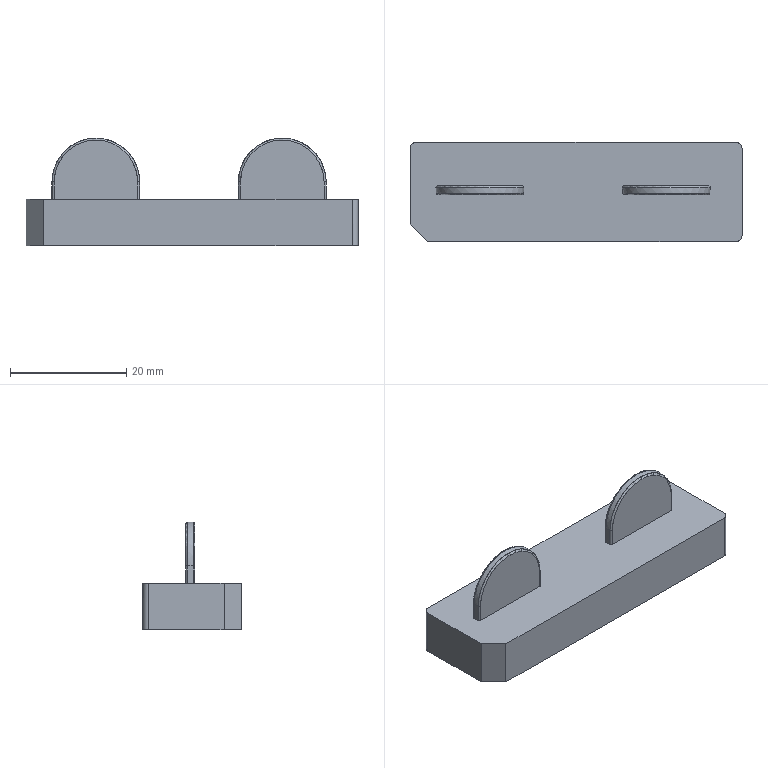NC program | PowerMill | posted by the shop | part box 57 x 17 x 18.538 mm
Lines 10661 to 11689 of 218548:
( TOOL ID   R1.5_1_1 )
( TOOL DIA. 3. TIP RAD 1.5 LENGTH 64.36 )
( Z = -9.391 )
T22 M6
T10
G91 G28 Z0
G0 G90 G54
M08
S22000 M3
X0 Y0 M8
G43 Z10.797 H22
X-10.444 Y-.885
Z-1.573
G1 Z-2.773 F1200
X-10.442 Y-.861 Z-2.798 F2000
X-10.437 Y-.836 Z-2.821
X-10.427 Y-.811 Z-2.843
X-10.415 Y-.785 Z-2.862
X-10.398 Y-.76 Z-2.88
X-10.379 Y-.736 Z-2.895
X-10.361 Y-.717 Z-2.906
X-10.33 Y-.685 Z-2.922
X-10.298 Y-.654 Z-2.94
X-10.264 Y-.62 Z-2.961
X-10.233 Y-.589 Z-2.981
X-10.203 Y-.559 Z-3.001
X-10.173 Y-.529 Z-3.023
X-10.16 Y-.515 Z-3.033
X-10.137 Y-.494 Z-3.049
X-10.111 Y-.474 Z-3.061
X-10.084 Y-.455 Z-3.07
X-10.054 Y-.438 Z-3.076
X-10.024 Y-.423 Z-3.079
X-9.992 Y-.409
X-9.966 Y-.4 Z-3.076
X-9.936 Y-.312 Z-3.091
X-9.969 Y-.324 Z-3.093
X-10. Y-.339
X-10.031 Y-.355 Z-3.089
X-10.059 Y-.372 Z-3.081
X-10.086 Y-.391 Z-3.071
X-10.111 Y-.411 Z-3.057
X-10.129 Y-.428 Z-3.044
X-10.159 Y-.458 Z-3.02
X-10.209 Y-.508 Z-2.981
X-10.266 Y-.565 Z-2.941
X-10.328 Y-.627 Z-2.901
X-10.39 Y-.689 Z-2.865
X-10.449 Y-.748 Z-2.835
X-10.504 Y-.803 Z-2.811
X-10.555 Y-.855 Z-2.791
X-10.606 Y-.905 Z-2.776
X-10.629 Y-.93 Z-2.767
X-10.649 Y-.956 Z-2.756
X-10.665 Y-.983 Z-2.742
X-10.679 Y-1.011 Z-2.726
X-10.689 Y-1.038 Z-2.708
X-10.696 Y-1.066 Z-2.689
X-10.699 Y-1.088 Z-2.672
X-10.809 Y-1.143 Z-2.618
X-10.805 Y-1.115 Z-2.638
X-10.797 Y-1.087 Z-2.656
X-10.786 Y-1.058 Z-2.672
X-10.771 Y-1.03 Z-2.686
X-10.753 Y-1.003 Z-2.697
X-10.733 Y-.977 Z-2.706
X-10.714 Y-.956 Z-2.712
X-10.662 Y-.904 Z-2.724
X-10.608 Y-.851 Z-2.741
X-10.552 Y-.795 Z-2.762
X-10.493 Y-.736 Z-2.788
X-10.432 Y-.675 Z-2.819
X-10.37 Y-.612 Z-2.855
X-10.306 Y-.549 Z-2.896
X-10.244 Y-.487 Z-2.94
X-10.186 Y-.428 Z-2.985
X-10.132 Y-.375 Z-3.031
X-10.113 Y-.356 Z-3.047
X-10.091 Y-.335 Z-3.064
X-10.066 Y-.316 Z-3.079
X-10.039 Y-.297 Z-3.09
X-10.011 Y-.28 Z-3.097
X-9.98 Y-.264 Z-3.102
X-9.949 Y-.249
X-9.923 Y-.239 Z-3.101
X-9.912 Y-.167 Z-3.109
X-9.944 Y-.181 Z-3.11
X-9.975 Y-.196 Z-3.109
X-10.005 Y-.213 Z-3.103
X-10.033 Y-.231 Z-3.095
X-10.059 Y-.25 Z-3.083
X-10.083 Y-.27 Z-3.067
X-10.1 Y-.286 Z-3.053
X-10.144 Y-.33 Z-3.013
X-10.205 Y-.391 Z-2.959
X-10.269 Y-.455 Z-2.908
X-10.332 Y-.518 Z-2.862
X-10.396 Y-.582 Z-2.82
X-10.459 Y-.645 Z-2.782
X-10.521 Y-.707 Z-2.75
X-10.582 Y-.768 Z-2.722
X-10.642 Y-.828 Z-2.698
X-10.701 Y-.887 Z-2.679
X-10.758 Y-.944 Z-2.664
X-10.814 Y-1. Z-2.653
X-10.837 Y-1.025 Z-2.647
X-10.858 Y-1.052 Z-2.639
X-10.875 Y-1.08 Z-2.628
X-10.889 Y-1.108 Z-2.615
X-10.9 Y-1.137 Z-2.599
X-10.908 Y-1.166 Z-2.582
X-10.911 Y-1.19 Z-2.567
X-11.011 Y-1.233 Z-2.525
X-11.005 Y-1.203 Z-2.542
X-10.997 Y-1.173 Z-2.558
X-10.984 Y-1.144 Z-2.571
X-10.969 Y-1.115 Z-2.582
X-10.951 Y-1.087 Z-2.591
X-10.93 Y-1.06 Z-2.597
X-10.911 Y-1.04 Z-2.6
X-10.864 Y-.993 Z-2.606
X-10.816 Y-.945 Z-2.614
X-10.763 Y-.892 Z-2.628
X-10.705 Y-.834 Z-2.646
X-10.643 Y-.772 Z-2.669
X-10.584 Y-.714 Z-2.695
X-10.533 Y-.662 Z-2.72
X-10.488 Y-.618 Z-2.745
X-10.445 Y-.574 Z-2.771
X-10.387 Y-.516 Z-2.809
X-10.329 Y-.459 Z-2.85
X-10.27 Y-.4 Z-2.896
X-10.206 Y-.336 Z-2.95
X-10.149 Y-.279 Z-3.001
X-10.096 Y-.226 Z-3.052
X-10.088 Y-.218 Z-3.059
X-10.067 Y-.198 Z-3.077
X-10.043 Y-.178 Z-3.092
X-10.016 Y-.159 Z-3.104
X-9.988 Y-.142 Z-3.112
X-9.958 Y-.125 Z-3.117
X-9.927 Y-.11 Z-3.119
X-9.901 Y-.099 Z-3.117
X-9.89 Y-.031 Z-3.119
X-9.921 Y-.045 Z-3.121
X-9.952 Y-.06 Z-3.119
X-9.982 Y-.077 Z-3.114
X-10.01 Y-.095 Z-3.105
X-10.036 Y-.114 Z-3.093
X-10.06 Y-.134 Z-3.078
X-10.078 Y-.151 Z-3.064
X-10.089 Y-.162 Z-3.053
X-10.138 Y-.211 Z-3.007
X-10.188 Y-.261 Z-2.961
X-10.242 Y-.315 Z-2.912
X-10.293 Y-.366 Z-2.868
X-10.344 Y-.417 Z-2.827
X-10.409 Y-.482 Z-2.779
X-10.473 Y-.546 Z-2.736
X-10.536 Y-.609 Z-2.698
X-10.599 Y-.672 Z-2.664
X-10.661 Y-.734 Z-2.635
X-10.722 Y-.795 Z-2.61
X-10.784 Y-.857 Z-2.589
X-10.842 Y-.914 Z-2.573
X-10.896 Y-.969 Z-2.562
X-10.948 Y-1.021 Z-2.554
X-10.998 Y-1.071 Z-2.551
X-11.022 Y-1.097 Z-2.548
X-11.042 Y-1.124 Z-2.543
X-11.06 Y-1.152 Z-2.535
X-11.075 Y-1.181 Z-2.524
X-11.087 Y-1.211 Z-2.511
X-11.096 Y-1.241 Z-2.497
X-11.1 Y-1.266 Z-2.483
X-11.185 Y-1.295 Z-2.446
X-11.179 Y-1.264 Z-2.462
X-11.169 Y-1.234 Z-2.475
X-11.157 Y-1.203 Z-2.486
X-11.141 Y-1.174 Z-2.494
X-11.122 Y-1.145 Z-2.5
X-11.101 Y-1.118 Z-2.504
X-11.082 Y-1.098
X-11.045 Y-1.061
X-11.008 Y-1.025 Z-2.507
X-10.966 Y-.982 Z-2.513
X-10.911 Y-.927 Z-2.523
X-10.867 Y-.883 Z-2.533
X-10.831 Y-.847 Z-2.543
X-10.795 Y-.811 Z-2.555
X-10.739 Y-.756 Z-2.576
X-10.685 Y-.701 Z-2.6
X-10.63 Y-.647 Z-2.627
X-10.576 Y-.592 Z-2.656
X-10.52 Y-.537 Z-2.69
X-10.464 Y-.48 Z-2.728
X-10.404 Y-.42 Z-2.771
X-10.34 Y-.357 Z-2.822
X-10.269 Y-.285 Z-2.883
X-10.186 Y-.202 Z-2.957
X-10.106 Y-.123 Z-3.032
X-10.068 Y-.084 Z-3.067
X-10.046 Y-.064 Z-3.085
X-10.022 Y-.044 Z-3.1
X-9.995 Y-.025 Z-3.111
X-9.967 Y-.007 Z-3.119
X-9.937 Y.009 Z-3.124
X-9.906 Y.024 Z-3.125
X-9.88 Y.035 Z-3.123
X-9.877 Y.095 Z-3.121
X-9.909 Y.081 Z-3.123
X-9.94 Y.066 Z-3.121
X-9.969 Y.049 Z-3.116
X-9.998 Y.031 Z-3.107
X-10.024 Y.011 Z-3.095
X-10.048 Y-.008 Z-3.08
X-10.065 Y-.025 Z-3.065
X-10.083 Y-.043 Z-3.048
X-10.126 Y-.086 Z-3.008
X-10.17 Y-.129 Z-2.968
X-10.213 Y-.173 Z-2.928
X-10.274 Y-.234 Z-2.873
X-10.329 Y-.288 Z-2.825
X-10.373 Y-.333 Z-2.788
X-10.417 Y-.377 Z-2.751
X-10.463 Y-.423 Z-2.716
X-10.509 Y-.469 Z-2.683
X-10.571 Y-.531 Z-2.642
X-10.635 Y-.595 Z-2.604
X-10.699 Y-.659 Z-2.571
X-10.763 Y-.723 Z-2.541
X-10.825 Y-.785 Z-2.517
X-10.886 Y-.846 Z-2.497
X-10.945 Y-.905 Z-2.481
X-11.002 Y-.962 Z-2.47
X-11.058 Y-1.018 Z-2.462
X-11.111 Y-1.071 Z-2.459
X-11.163 Y-1.123 Z-2.46
X-11.187 Y-1.149 Z-2.459
X-11.208 Y-1.176 Z-2.455
X-11.226 Y-1.205 Z-2.449
X-11.241 Y-1.234 Z-2.44
X-11.253 Y-1.264 Z-2.429
X-11.262 Y-1.295 Z-2.416
X-11.267 Y-1.32 Z-2.404
X-11.349 Y-1.346 Z-2.368
X-11.343 Y-1.315 Z-2.382
X-11.333 Y-1.284 Z-2.394
X-11.32 Y-1.253 Z-2.403
X-11.304 Y-1.224 Z-2.411
X-11.285 Y-1.195 Z-2.415
X-11.263 Y-1.168 Z-2.417
X-11.244 Y-1.147
X-11.194 Y-1.098 Z-2.414
X-11.143 Y-1.046 Z-2.415
X-11.089 Y-.992 Z-2.419
X-11.032 Y-.935 Z-2.428
X-10.974 Y-.877 Z-2.441
X-10.913 Y-.816 Z-2.459
X-10.851 Y-.754 Z-2.481
X-10.787 Y-.69 Z-2.508
X-10.723 Y-.626 Z-2.538
X-10.66 Y-.563 Z-2.573
X-10.613 Y-.517 Z-2.6
X-10.565 Y-.468 Z-2.632
X-10.517 Y-.42 Z-2.667
X-10.469 Y-.372 Z-2.703
X-10.417 Y-.32 Z-2.745
X-10.356 Y-.259 Z-2.796
X-10.281 Y-.184 Z-2.862
X-10.183 Y-.086 Z-2.95
X-10.113 Y-.016 Z-3.014
X-10.062 Y.035 Z-3.062
X-10.04 Y.055 Z-3.08
X-10.016 Y.074 Z-3.094
X-9.99 Y.093 Z-3.106
X-9.961 Y.111 Z-3.114
X-9.931 Y.128 Z-3.119
X-9.9 Y.143 Z-3.12
X-9.874 Y.154 Z-3.118
X-9.872 Y.213 Z-3.116
X-9.904 Y.199 Z-3.118
X-9.935 Y.184 Z-3.116
X-9.964 Y.167 Z-3.11
X-9.992 Y.149 Z-3.102
X-10.018 Y.13 Z-3.089
X-10.042 Y.11 Z-3.074
X-10.06 Y.094 Z-3.059
X-10.106 Y.048 Z-3.016
X-10.156 Y-.003 Z-2.969
X-10.207 Y-.053 Z-2.923
X-10.257 Y-.104 Z-2.878
X-10.309 Y-.155 Z-2.833
X-10.368 Y-.214 Z-2.781
X-10.419 Y-.266 Z-2.737
X-10.471 Y-.318 Z-2.694
X-10.524 Y-.37 Z-2.652
X-10.577 Y-.423 Z-2.613
X-10.641 Y-.488 Z-2.569
X-10.706 Y-.553 Z-2.53
X-10.772 Y-.618 Z-2.494
X-10.838 Y-.684 Z-2.462
X-10.89 Y-.736 Z-2.44
X-10.945 Y-.792 Z-2.42
X-11.006 Y-.852 Z-2.402
X-11.067 Y-.914 Z-2.388
X-11.125 Y-.972 Z-2.378
X-11.18 Y-1.026 Z-2.372
X-11.23 Y-1.076 Z-2.37
X-11.276 Y-1.122 Z-2.371
X-11.321 Y-1.167 Z-2.376
X-11.344 Y-1.193 Z-2.377
X-11.365 Y-1.22 Z-2.376
X-11.384 Y-1.249 Z-2.372
X-11.399 Y-1.279 Z-2.365
X-11.412 Y-1.31 Z-2.356
X-11.421 Y-1.342 Z-2.344
X-11.427 Y-1.367 Z-2.334
X-11.502 Y-1.386 Z-2.297
X-11.496 Y-1.355 Z-2.31
X-11.485 Y-1.323 Z-2.32
X-11.472 Y-1.292 Z-2.329
X-11.456 Y-1.262 Z-2.334
X-11.437 Y-1.234 Z-2.337
X-11.415 Y-1.207
X-11.396 Y-1.186 Z-2.336
X-11.35 Y-1.14 Z-2.33
X-11.303 Y-1.093 Z-2.327
X-11.251 Y-1.041 Z-2.328
X-11.195 Y-.985 Z-2.333
X-11.135 Y-.925 Z-2.341
X-11.073 Y-.864 Z-2.354
X-11.016 Y-.806 Z-2.37
X-10.963 Y-.753 Z-2.387
X-10.915 Y-.705 Z-2.406
X-10.855 Y-.645 Z-2.433
X-10.794 Y-.584 Z-2.464
X-10.729 Y-.519 Z-2.501
X-10.663 Y-.453 Z-2.542
X-10.603 Y-.393 Z-2.584
X-10.547 Y-.338 Z-2.626
X-10.493 Y-.283 Z-2.671
X-10.367 Y-.157 Z-2.777
X-10.24 Y-.03 Z-2.888
X-10.111 Y.099 Z-3.006
X-10.057 Y.153 Z-3.057
X-10.035 Y.173 Z-3.074
X-10.011 Y.193 Z-3.089
X-9.984 Y.212 Z-3.101
X-9.956 Y.23 Z-3.109
X-9.926 Y.246 Z-3.113
X-9.895 Y.261 Z-3.115
X-9.869 Y.272 Z-3.113
X-9.867 Y.331 Z-3.111
X-9.898 Y.318 Z-3.113
X-9.929 Y.302 Z-3.111
X-9.959 Y.285 Z-3.105
X-9.987 Y.267 Z-3.096
X-10.013 Y.248 Z-3.084
X-10.037 Y.228 Z-3.068
X-10.054 Y.212 Z-3.054
X-10.07 Y.197 Z-3.039
X-10.121 Y.145 Z-2.991
X-10.172 Y.094 Z-2.944
X-10.224 Y.042 Z-2.897
X-10.276 Y-.01 Z-2.851
X-10.347 Y-.081 Z-2.789
X-10.427 Y-.161 Z-2.72
X-10.486 Y-.219 Z-2.671
X-10.539 Y-.272 Z-2.628
X-10.592 Y-.326 Z-2.585
X-10.646 Y-.38 Z-2.545
X-10.693 Y-.426 Z-2.511
X-10.756 Y-.489 Z-2.47
X-10.82 Y-.553 Z-2.433
X-10.884 Y-.618 Z-2.399
X-10.948 Y-.682 Z-2.37
X-11.012 Y-.745 Z-2.345
X-11.074 Y-.808 Z-2.325
X-11.135 Y-.869 Z-2.309
X-11.195 Y-.928 Z-2.297
X-11.253 Y-.987 Z-2.289
X-11.31 Y-1.043 Z-2.285
X-11.365 Y-1.098
X-11.418 Y-1.152 Z-2.289
X-11.47 Y-1.204 Z-2.297
X-11.494 Y-1.229 Z-2.299
X-11.515 Y-1.257
X-11.533 Y-1.286 Z-2.296
X-11.549 Y-1.316 Z-2.291
X-11.562 Y-1.347 Z-2.283
X-11.572 Y-1.379 Z-2.272
X-11.577 Y-1.404 Z-2.262
X-11.652 Y-1.422 Z-2.234
X-11.644 Y-1.39 Z-2.245
X-11.634 Y-1.358 Z-2.254
X-11.62 Y-1.327 Z-2.26
X-11.604 Y-1.297 Z-2.264
X-11.584 Y-1.268 Z-2.265
X-11.563 Y-1.241 Z-2.263
X-11.544 Y-1.221 Z-2.26
X-11.506 Y-1.183 Z-2.252
X-11.467 Y-1.144 Z-2.247
X-11.422 Y-1.099 Z-2.244
X-11.369 Y-1.046 Z-2.243
X-11.314 Y-.991 Z-2.247
X-11.268 Y-.945 Z-2.252
X-11.228 Y-.904 Z-2.258
X-11.168 Y-.845 Z-2.271
X-11.107 Y-.784 Z-2.288
X-11.044 Y-.721 Z-2.309
X-10.981 Y-.658 Z-2.335
X-10.915 Y-.592 Z-2.366
X-10.847 Y-.524 Z-2.402
X-10.777 Y-.454 Z-2.444
X-10.751 Y-.428 Z-2.46
X-10.725 Y-.402 Z-2.478
X-10.7 Y-.377 Z-2.497
X-10.675 Y-.352 Z-2.516
X-10.646 Y-.323 Z-2.538
X-10.61 Y-.287 Z-2.567
X-10.558 Y-.235 Z-2.608
X-10.515 Y-.192 Z-2.643
X-10.483 Y-.159 Z-2.669
X-10.457 Y-.134 Z-2.69
X-10.432 Y-.109 Z-2.711
X-10.407 Y-.084 Z-2.731
X-10.383 Y-.06 Z-2.753
X-10.239 Y.084 Z-2.879
X-10.122 Y.201 Z-2.985
X-10.052 Y.271 Z-3.051
X-10.03 Y.292 Z-3.069
X-10.006 Y.311 Z-3.083
X-9.979 Y.33 Z-3.095
X-9.951 Y.348 Z-3.103
X-9.921 Y.365 Z-3.108
X-9.89 Y.38 Z-3.109
X-9.864 Y.391 Z-3.107
X-9.861 Y.45 Z-3.103
X-9.893 Y.436 Z-3.105
X-9.924 Y.421 Z-3.104
X-9.953 Y.404 Z-3.098
X-9.982 Y.386 Z-3.09
X-10.008 Y.367 Z-3.078
X-10.032 Y.347 Z-3.063
X-10.049 Y.331 Z-3.048
X-10.162 Y.218 Z-2.943
X-10.293 Y.086 Z-2.826
X-10.43 Y-.05 Z-2.708
X-10.571 Y-.192 Z-2.591
X-10.636 Y-.256 Z-2.539
X-10.702 Y-.323 Z-2.488
X-10.772 Y-.392 Z-2.439
X-10.838 Y-.459 Z-2.395
X-10.902 Y-.522 Z-2.357
X-10.963 Y-.583 Z-2.324
X-11.025 Y-.646 Z-2.295
X-11.073 Y-.694 Z-2.275
X-11.124 Y-.744 Z-2.257
X-11.179 Y-.799 Z-2.24
X-11.238 Y-.858 Z-2.225
X-11.3 Y-.921 Z-2.213
X-11.361 Y-.981 Z-2.206
X-11.419 Y-1.039 Z-2.202
X-11.473 Y-1.094 Z-2.203
X-11.524 Y-1.145 Z-2.206
X-11.572 Y-1.192 Z-2.213
X-11.617 Y-1.237 Z-2.224
X-11.64 Y-1.263 Z-2.228
X-11.661 Y-1.29 Z-2.229
X-11.68 Y-1.319 Z-2.228
X-11.696 Y-1.35 Z-2.224
X-11.709 Y-1.381 Z-2.218
X-11.719 Y-1.413 Z-2.209
X-11.725 Y-1.439 Z-2.2
X-11.796 Y-1.452 Z-2.167
X-11.788 Y-1.42 Z-2.177
X-11.777 Y-1.388 Z-2.186
X-11.763 Y-1.357 Z-2.191
X-11.747 Y-1.327 Z-2.194
X-11.728 Y-1.298 Z-2.195
X-11.706 Y-1.271 Z-2.192
X-11.687 Y-1.251 Z-2.188
X-11.638 Y-1.202 Z-2.176
X-11.587 Y-1.151 Z-2.168
X-11.534 Y-1.098 Z-2.163
X-11.478 Y-1.042 Z-2.162
X-11.421 Y-.984 Z-2.164
X-11.361 Y-.925 Z-2.171
X-11.3 Y-.864 Z-2.182
X-11.238 Y-.802 Z-2.197
X-11.176 Y-.739 Z-2.216
X-11.114 Y-.678 Z-2.238
X-11.065 Y-.629 Z-2.259
X-11.01 Y-.574 Z-2.285
X-10.956 Y-.519 Z-2.313
X-10.902 Y-.466 Z-2.344
X-10.849 Y-.412 Z-2.377
X-10.787 Y-.35 Z-2.42
X-10.732 Y-.296 Z-2.46
X-10.681 Y-.245 Z-2.5
X-10.63 Y-.194 Z-2.54
X-10.579 Y-.143 Z-2.58
X-10.445 Y-.009 Z-2.69
X-10.312 Y.124 Z-2.804
X-10.18 Y.256 Z-2.921
X-10.05 Y.387 Z-3.043
X-10.046 Y.39 Z-3.045
X-10.025 Y.41 Z-3.063
X-10. Y.43 Z-3.078
X-9.974 Y.448 Z-3.09
X-9.945 Y.466 Z-3.098
X-9.915 Y.483 Z-3.103
X-9.884 Y.498 Z-3.104
X-9.859 Y.509 Z-3.102
X-9.856 Y.569 Z-3.098
X-9.888 Y.555 Z-3.1
X-9.918 Y.539 Z-3.098
X-9.948 Y.522 Z-3.093
X-9.976 Y.504 Z-3.084
X-10.003 Y.485 Z-3.072
X-10.026 Y.465 Z-3.057
X-10.044 Y.449 Z-3.043
X-10.135 Y.357 Z-2.957
X-10.266 Y.227 Z-2.839
X-10.396 Y.097 Z-2.727
X-10.525 Y-.032 Z-2.619
X-10.63 Y-.138 Z-2.535
X-10.709 Y-.216 Z-2.473
X-10.775 Y-.283 Z-2.423
X-10.834 Y-.341 Z-2.381
X-10.888 Y-.395 Z-2.343
X-10.943 Y-.451 Z-2.308
X-10.999 Y-.506 Z-2.275
X-11.065 Y-.572 Z-2.241
X-11.13 Y-.638 Z-2.211
X-11.194 Y-.702 Z-2.186
X-11.258 Y-.765 Z-2.165
X-11.32 Y-.827 Z-2.148
X-11.381 Y-.888 Z-2.136
X-11.441 Y-.948 Z-2.127
X-11.5 Y-1.008 Z-2.123
X-11.559 Y-1.066 Z-2.122
X-11.613 Y-1.12 Z-2.125
X-11.664 Y-1.171 Z-2.131
X-11.712 Y-1.219 Z-2.141
X-11.757 Y-1.264 Z-2.153
X-11.78 Y-1.289 Z-2.159
X-11.801 Y-1.317 Z-2.162
X-11.82 Y-1.346
X-11.836 Y-1.376 Z-2.159
X-11.849 Y-1.408 Z-2.154
X-11.859 Y-1.44 Z-2.146
X-11.866 Y-1.466 Z-2.138
X-11.935 Y-1.478 Z-2.11
X-11.927 Y-1.446 Z-2.119
X-11.916 Y-1.414 Z-2.126
X-11.902 Y-1.382 Z-2.13
X-11.885 Y-1.352 Z-2.131
X-11.866 Y-1.323 Z-2.129
X-11.845 Y-1.297 Z-2.125
X-11.826 Y-1.276 Z-2.12
X-11.789 Y-1.239 Z-2.108
X-11.751 Y-1.202 Z-2.099
X-11.707 Y-1.158 Z-2.091
X-11.656 Y-1.107 Z-2.086
X-11.597 Y-1.048 Z-2.083
X-11.547 Y-.998 Z-2.084
X-11.505 Y-.955 Z-2.086
X-11.467 Y-.917 Z-2.091
X-11.429 Y-.88 Z-2.096
X-11.367 Y-.818 Z-2.109
X-11.304 Y-.754 Z-2.127
X-11.239 Y-.689 Z-2.148
X-11.172 Y-.623 Z-2.174
X-11.104 Y-.555 Z-2.205
X-11.046 Y-.496 Z-2.235
X-11. Y-.451 Z-2.261
X-10.955 Y-.405 Z-2.29
X-10.91 Y-.361 Z-2.32
X-10.861 Y-.312 Z-2.354
X-10.801 Y-.252 Z-2.398
X-10.716 Y-.166 Z-2.463
X-10.655 Y-.105 Z-2.511
X-10.606 Y-.057 Z-2.549
X-10.563 Y-.014 Z-2.584
X-10.52 Y.029 Z-2.619
X-10.478 Y.072 Z-2.654
X-10.354 Y.196 Z-2.758
X-10.228 Y.321 Z-2.868
X-10.1 Y.449 Z-2.985
X-10.041 Y.508 Z-3.04
X-10.02 Y.528 Z-3.058
X-9.995 Y.548 Z-3.072
X-9.969 Y.567 Z-3.084
X-9.94 Y.585 Z-3.092
X-9.91 Y.601 Z-3.097
X-9.879 Y.617 Z-3.098
X-9.853 Y.628 Z-3.096
X-9.851 Y.687 Z-3.094
X-9.882 Y.673 Z-3.095
X-9.913 Y.658 Z-3.093
X-9.943 Y.641 Z-3.088
X-9.971 Y.623 Z-3.079
X-9.997 Y.604 Z-3.067
X-10.021 Y.584 Z-3.052
X-10.039 Y.567 Z-3.037
X-10.089 Y.517 Z-2.989
X-10.198 Y.408 Z-2.89
X-10.333 Y.273 Z-2.772
X-10.428 Y.178 Z-2.69
X-10.53 Y.076 Z-2.605
X-10.655 Y-.049 Z-2.506
X-10.701 Y-.095 Z-2.47
X-10.748 Y-.142 Z-2.434
X-10.808 Y-.202 Z-2.388
X-10.876 Y-.27 Z-2.338
X-10.925 Y-.32 Z-2.302
X-10.973 Y-.367 Z-2.27
X-11.021 Y-.415 Z-2.239
X-11.07 Y-.464 Z-2.211
X-11.141 Y-.535 Z-2.174
X-11.209 Y-.603 Z-2.142
X-11.275 Y-.669 Z-2.115
X-11.34 Y-.734 Z-2.092
X-11.403 Y-.797 Z-2.074
X-11.464 Y-.858 Z-2.061
X-11.525 Y-.919 Z-2.051
X-11.564 Y-.958 Z-2.047
X-11.608 Y-1.002 Z-2.045
X-11.659 Y-1.053
X-11.716 Y-1.111 Z-2.048
X-11.77 Y-1.164 Z-2.054
X-11.816 Y-1.21 Z-2.063
X-11.856 Y-1.25 Z-2.073
X-11.894 Y-1.289 Z-2.087
X-11.917 Y-1.314 Z-2.093
X-11.938 Y-1.341 Z-2.098
X-11.957 Y-1.37 Z-2.099
X-11.973 Y-1.4 Z-2.098
X-11.987 Y-1.432 Z-2.094
X-11.997 Y-1.464 Z-2.087
X-12.004 Y-1.49 Z-2.08
X-12.072 Y-1.502 Z-2.051
X-12.064 Y-1.47 Z-2.059
X-12.053 Y-1.438 Z-2.065
X-12.039 Y-1.406 Z-2.068
X-12.022 Y-1.376 Z-2.069
X-12.003 Y-1.347 Z-2.066
X-11.981 Y-1.32 Z-2.061
X-11.963 Y-1.3 Z-2.055
X-11.923 Y-1.261 Z-2.041
X-11.882 Y-1.22 Z-2.029
X-11.835 Y-1.173 Z-2.019
X-11.782 Y-1.119 Z-2.012
X-11.725 Y-1.062 Z-2.007
X-11.674 Y-1.012 Z-2.006
X-11.631 Y-.969 Z-2.008
X-11.59 Y-.928 Z-2.011
X-11.527 Y-.865 Z-2.02
X-11.464 Y-.801 Z-2.033
X-11.399 Y-.737 Z-2.05
X-11.335 Y-.672 Z-2.071
X-11.27 Y-.607 Z-2.097
X-11.204 Y-.542 Z-2.126
X-11.139 Y-.476 Z-2.16
X-11.073 Y-.41 Z-2.199
X-11.015 Y-.352 Z-2.236
X-10.944 Y-.282 Z-2.284
X-10.874 Y-.211 Z-2.335
X-10.804 Y-.141 Z-2.387
X-10.727 Y-.064 Z-2.445
X-10.658 Y.005 Z-2.499
X-10.589 Y.074 Z-2.553
X-10.52 Y.142 Z-2.608
X-10.452 Y.211 Z-2.664
X-10.384 Y.278 Z-2.722
X-10.249 Y.414 Z-2.84
X-10.117 Y.545 Z-2.958
X-10.038 Y.624 Z-3.032
X-10.016 Y.645 Z-3.05
X-9.992 Y.664 Z-3.065
X-9.965 Y.683 Z-3.076
X-9.937 Y.701 Z-3.084
X-9.907 Y.718 Z-3.089
X-9.876 Y.733 Z-3.09
X-9.85 Y.744 Z-3.088
X-9.853 Y.797
X-9.885 Y.783 Z-3.089
X-9.916 Y.768 Z-3.087
X-9.945 Y.751 Z-3.081
X-9.973 Y.733 Z-3.071
X-9.999 Y.715 Z-3.058
X-10.023 Y.695 Z-3.042
X-10.04 Y.679 Z-3.027
X-10.072 Y.647 Z-2.995
X-10.107 Y.612 Z-2.962
X-10.142 Y.578 Z-2.93
X-10.176 Y.543 Z-2.899
X-10.231 Y.488 Z-2.85
X-10.272 Y.447 Z-2.814
X-10.307 Y.412 Z-2.783
X-10.342 Y.377 Z-2.752
X-10.378 Y.341 Z-2.722
X-10.495 Y.224 Z-2.624
X-10.619 Y.1 Z-2.524
X-10.744 Y-.025 Z-2.427
X-10.87 Y-.151 Z-2.333
X-10.997 Y-.278 Z-2.242
X-11.056 Y-.337 Z-2.201
X-11.118 Y-.399 Z-2.162
X-11.183 Y-.464 Z-2.124
X-11.251 Y-.532 Z-2.09
X-11.319 Y-.6 Z-2.059
X-11.386 Y-.666 Z-2.033
X-11.45 Y-.731 Z-2.012
X-11.513 Y-.794 Z-1.995
X-11.573 Y-.854 Z-1.983
X-11.619 Y-.9 Z-1.976
X-11.667 Y-.948 Z-1.971
X-11.721 Y-1.002 Z-1.969
X-11.78 Y-1.061 Z-1.97
X-11.838 Y-1.119 Z-1.975
X-11.893 Y-1.174 Z-1.983
X-11.943 Y-1.224 Z-1.994
X-11.988 Y-1.269 Z-2.007
X-12.031 Y-1.311 Z-2.023
X-12.053 Y-1.336 Z-2.031
X-12.074 Y-1.364 Z-2.035
X-12.093 Y-1.393 Z-2.037
X-12.109 Y-1.423
X-12.123 Y-1.455 Z-2.033
X-12.134 Y-1.487 Z-2.027
X-12.14 Y-1.513 Z-2.02
X-12.207 Y-1.524 Z-1.99
X-12.199 Y-1.491 Z-1.998
X-12.187 Y-1.459 Z-2.004
X-12.173 Y-1.427 Z-2.007
X-12.156 Y-1.397
X-12.137 Y-1.368 Z-2.004
X-12.116 Y-1.342 Z-1.999
X-12.097 Y-1.322 Z-1.992
X-12.047 Y-1.271 Z-1.973
X-11.995 Y-1.219 Z-1.958
X-11.941 Y-1.165 Z-1.946
X-11.886 Y-1.11 Z-1.937
X-11.828 Y-1.053 Z-1.933
X-11.77 Y-.994 Z-1.932
X-11.709 Y-.934 Z-1.935
X-11.647 Y-.872 Z-1.942
X-11.584 Y-.809 Z-1.954
X-11.52 Y-.744 Z-1.969
X-11.455 Y-.679 Z-1.989
X-11.39 Y-.615 Z-2.012
X-11.325 Y-.55 Z-2.04
X-11.259 Y-.484 Z-2.072
X-11.192 Y-.416 Z-2.109
X-11.143 Y-.367 Z-2.139
X-11.094 Y-.319 Z-2.171
X-11.046 Y-.271 Z-2.203
X-10.998 Y-.223 Z-2.237
X-10.947 Y-.171 Z-2.273
X-10.878 Y-.102 Z-2.323
X-10.807 Y-.031 Z-2.375
X-10.755 Y.02 Z-2.414
X-10.708 Y.067 Z-2.45
X-10.661 Y.114 Z-2.486
X-10.614 Y.161 Z-2.522
X-10.576 Y.199 Z-2.553
X-10.539 Y.237 Z-2.583
X-10.501 Y.275 Z-2.614
X-10.463 Y.312 Z-2.646
X-10.424 Y.352 Z-2.679
X-10.375 Y.4 Z-2.72
X-10.309 Y.466 Z-2.776
X-10.246 Y.53 Z-2.831
X-10.199 Y.577 Z-2.873
X-10.161 Y.615 Z-2.908
X-10.124 Y.651 Z-2.941
X-10.088 Y.687 Z-2.976
X-10.053 Y.723 Z-3.012
X-10.043 Y.732 Z-3.022
X-10.023 Y.752 Z-3.041
X-9.999 Y.771 Z-3.058
X-9.973 Y.789 Z-3.071
X-9.945 Y.807 Z-3.081
X-9.915 Y.824 Z-3.088
X-9.885 Y.839 Z-3.091
X-9.859 Y.851
X-9.865 Y.905 Z-3.088
X-9.896 Y.89
X-9.927 Y.874 Z-3.084
X-9.956 Y.856 Z-3.077
X-9.983 Y.838 Z-3.066
X-10.008 Y.819 Z-3.052
X-10.031 Y.8 Z-3.035
X-10.048 Y.784 Z-3.018
X-10.072 Y.76 Z-2.992
X-10.122 Y.71 Z-2.941
X-10.184 Y.649 Z-2.883
X-10.232 Y.6 Z-2.839
X-10.289 Y.543 Z-2.788
X-10.368 Y.464 Z-2.72
X-10.451 Y.381 Z-2.651
X-10.577 Y.255 Z-2.547
X-10.681 Y.151 Z-2.466
X-10.785 Y.047 Z-2.387
X-10.907 Y-.075 Z-2.296
X-11.022 Y-.19 Z-2.215
X-11.129 Y-.296 Z-2.142
X-11.193 Y-.361 Z-2.101
X-11.258 Y-.426 Z-2.062
X-11.324 Y-.492 Z-2.027
X-11.39 Y-.558 Z-1.996
X-11.456 Y-.624 Z-1.969
X-11.522 Y-.69 Z-1.946
X-11.587 Y-.755 Z-1.928
X-11.651 Y-.819 Z-1.914
X-11.713 Y-.881 Z-1.904
X-11.775 Y-.943 Z-1.898
X-11.835 Y-1.003 Z-1.896
X-11.894 Y-1.062 Z-1.898
X-11.952 Y-1.12 Z-1.903
X-12.007 Y-1.175 Z-1.913
X-12.061 Y-1.229 Z-1.926
X-12.113 Y-1.281 Z-1.942
X-12.163 Y-1.331 Z-1.962
X-12.186 Y-1.356 Z-1.97
X-12.207 Y-1.383 Z-1.975
X-12.226 Y-1.412 Z-1.978
X-12.242 Y-1.442
X-12.256 Y-1.474 Z-1.974
X-12.267 Y-1.506 Z-1.969
X-12.273 Y-1.533 Z-1.962
X-12.338 Y-1.541 Z-1.937
X-12.33 Y-1.509 Z-1.944
X-12.318 Y-1.477 Z-1.949
X-12.304 Y-1.445 Z-1.951
X-12.287 Y-1.415 Z-1.95
X-12.268 Y-1.386 Z-1.946
X-12.247 Y-1.36 Z-1.94
X-12.229 Y-1.34 Z-1.932
X-12.182 Y-1.293 Z-1.913
X-12.133 Y-1.244 Z-1.896
X-12.08 Y-1.192 Z-1.882
X-12.025 Y-1.136 Z-1.871
X-11.967 Y-1.078 Z-1.864
X-11.908 Y-1.019 Z-1.86
X-11.847 Y-.958 Z-1.861
X-11.788 Y-.899 Z-1.865
X-11.737 Y-.849 Z-1.871
X-11.674 Y-.785 Z-1.883
X-11.61 Y-.721 Z-1.899
X-11.544 Y-.655 Z-1.919
X-11.477 Y-.588 Z-1.944
X-11.41 Y-.521 Z-1.973
X-11.341 Y-.452 Z-2.007
X-11.272 Y-.384 Z-2.045
X-11.204 Y-.315 Z-2.087
X-11.135 Y-.246 Z-2.133
X-10.977 Y-.089 Z-2.242
X-10.837 Y.052 Z-2.344
X-10.708 Y.181 Z-2.44
X-10.588 Y.3 Z-2.534
X-10.47 Y.418 Z-2.63
X-10.334 Y.555 Z-2.744
X-10.282 Y.606 Z-2.788
X-10.231 Y.657 Z-2.835
X-10.181 Y.708 Z-2.882
X-10.123 Y.765 Z-2.94
X-10.075 Y.814 Z-2.992
X-10.054 Y.835 Z-3.016
X-10.033 Y.854 Z-3.036
X-10.01 Y.873 Z-3.053
X-9.985 Y.892 Z-3.067
X-9.957 Y.91 Z-3.078
X-9.928 Y.928 Z-3.085
X-9.898 Y.944 Z-3.088
X-9.873 Y.956
X-9.882 Y1.007 Z-3.091
X-9.912 Y.991 Z-3.09
X-9.942 Y.974 Z-3.086
X-9.97 Y.957 Z-3.077
X-9.997 Y.938 Z-3.065
X-10.022 Y.919 Z-3.05
X-10.044 Y.9 Z-3.031
X-10.06 Y.885 Z-3.014
X-10.075 Y.871 Z-2.997
X-10.119 Y.827 Z-2.947
X-10.164 Y.782 Z-2.9
X-10.222 Y.723 Z-2.842
X-10.276 Y.669 Z-2.791
X-10.324 Y.621 Z-2.748
X-10.372 Y.573 Z-2.706
X-10.508 Y.437 Z-2.593
X-10.646 Y.299 Z-2.483
X-10.787 Y.158 Z-2.376
X-10.93 Y.015 Z-2.271
X-11.076 Y-.131 Z-2.168
X-11.224 Y-.279 Z-2.069
X-11.287 Y-.341 Z-2.029
X-11.352 Y-.406 Z-1.991
X-11.419 Y-.474 Z-1.956
X-11.487 Y-.542 Z-1.924
X-11.555 Y-.61 Z-1.897
X-11.622 Y-.677 Z-1.874
X-11.687 Y-.742 Z-1.856
X-11.75 Y-.805 Z-1.842
X-11.811 Y-.866 Z-1.833
X-11.865 Y-.92 Z-1.827
X-11.922 Y-.977 Z-1.825
X-11.982 Y-1.037 Z-1.826
X-12.042 Y-1.096 Z-1.832
X-12.099 Y-1.154 Z-1.84
X-12.153 Y-1.207 Z-1.852
X-12.203 Y-1.258 Z-1.867
X-12.249 Y-1.304 Z-1.884
X-12.293 Y-1.348 Z-1.904
X-12.316 Y-1.372 Z-1.914
X-12.336 Y-1.399 Z-1.92
X-12.355 Y-1.428 Z-1.924
X-12.371 Y-1.459 Z-1.925
X-12.385 Y-1.49 Z-1.923
X-12.396 Y-1.523 Z-1.919
X-12.403 Y-1.549 Z-1.913
X-12.47 Y-1.559 Z-1.887
X-12.461 Y-1.526 Z-1.894
X-12.449 Y-1.494 Z-1.898
X-12.435 Y-1.462 Z-1.899
X-12.418 Y-1.432 Z-1.897
X-12.399 Y-1.404 Z-1.892
X-12.378 Y-1.377 Z-1.885
X-12.359 Y-1.357 Z-1.877
X-12.312 Y-1.31 Z-1.854
X-12.263 Y-1.261 Z-1.835
X-12.211 Y-1.209 Z-1.819
X-12.157 Y-1.155 Z-1.807
X-12.101 Y-1.099 Z-1.798
X-12.043 Y-1.041 Z-1.792
X-11.983 Y-.981 Z-1.791
X-11.921 Y-.919 Z-1.793
X-11.857 Y-.856 Z-1.799
X-11.793 Y-.791 Z-1.809
X-11.728 Y-.727 Z-1.823
X-11.664 Y-.663 Z-1.841
X-11.603 Y-.601 Z-1.862
X-11.54 Y-.538 Z-1.887
X-11.475 Y-.473 Z-1.917
X-11.407 Y-.405 Z-1.953
X-11.333 Y-.332 Z-1.995
X-11.254 Y-.252 Z-2.045
X-11.164 Y-.162 Z-2.104
X-11.024 Y-.022 Z-2.2
X-10.895 Y.107 Z-2.291
X-10.757 Y.245 Z-2.393
X-10.617 Y.385 Z-2.502
X-10.473 Y.529 Z-2.618
X-10.401 Y.6 Z-2.677
X-10.328 Y.674 Z-2.742
X-10.257 Y.745 Z-2.808
X-10.193 Y.809 Z-2.873
X-10.135 Y.867 Z-2.935
X-10.083 Y.919 Z-2.995
X-10.068 Y.934 Z-3.014
X-10.048 Y.953 Z-3.035
X-10.025 Y.972 Z-3.053
X-10.001 Y.991 Z-3.068
X-9.975 Y1.008 Z-3.079
X-9.947 Y1.026 Z-3.087
X-9.917 Y1.044 Z-3.091
X-9.891 Y1.058 Z-3.092
X-9.901 Y1.105 Z-3.091
X-9.933 Y1.087 Z-3.089
X-9.963 Y1.069 Z-3.084
X-9.99 Y1.052 Z-3.075
X-10.015 Y1.034 Z-3.064
X-10.04 Y1.015 Z-3.048
X-10.062 Y.996 Z-3.029
X-10.078 Y.981 Z-3.012
X-10.098 Y.96 Z-2.987
X-10.162 Y.896 Z-2.911
X-10.227 Y.832 Z-2.84
X-10.291 Y.768 Z-2.775
X-10.355 Y.703 Z-2.714
X-10.419 Y.639 Z-2.657
X-10.527 Y.531 Z-2.568
X-10.66 Y.398 Z-2.463
X-10.796 Y.262 Z-2.359
X-10.935 Y.124 Z-2.258
X-11.064 Y-.006 Z-2.167
X-11.18 Y-.121 Z-2.09
X-11.293 Y-.235 Z-2.015
X-11.375 Y-.317 Z-1.963
X-11.445 Y-.386 Z-1.922
X-11.508 Y-.449 Z-1.889
X-11.568 Y-.509 Z-1.861
X-11.637 Y-.578 Z-1.834
X-11.704 Y-.646 Z-1.81
X-11.771 Y-.712 Z-1.791
X-11.836 Y-.778 Z-1.776
X-11.9 Y-.842 Z-1.765
X-11.963 Y-.905 Z-1.759
X-12.025 Y-.967 Z-1.756
X-12.075 Y-1.016 Z-1.757
X-12.128 Y-1.07 Z-1.761
X-12.186 Y-1.128 Z-1.769
X-12.243 Y-1.184 Z-1.781
X-12.295 Y-1.236 Z-1.795
X-12.341 Y-1.282 Z-1.811
X-12.382 Y-1.324 Z-1.828
X-12.422 Y-1.364 Z-1.849
X-12.444 Y-1.388 Z-1.859
X-12.465 Y-1.415 Z-1.867
X-12.483 Y-1.443 Z-1.872
X-12.5 Y-1.474 Z-1.874
X-12.514 Y-1.506 Z-1.873
X-12.525 Y-1.538 Z-1.869
X-12.532 Y-1.565 Z-1.864
X-12.597 Y-1.572 Z-1.838
X-12.588 Y-1.539 Z-1.844
X-12.576 Y-1.507 Z-1.847
X-12.561 Y-1.476
X-12.544 Y-1.445 Z-1.844
X-12.525 Y-1.417 Z-1.839
X-12.505 Y-1.391 Z-1.83
X-12.486 Y-1.371 Z-1.822
X-12.444 Y-1.329 Z-1.8
X-12.4 Y-1.285 Z-1.78
X-12.351 Y-1.236 Z-1.763